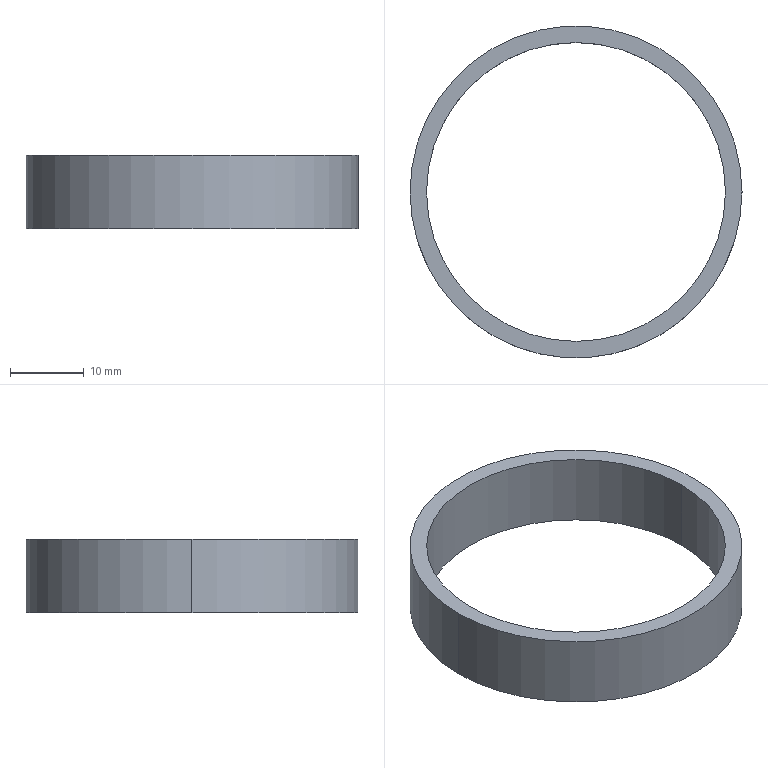Part | SolidWorks | features Extrusion 1 | 1 solid | 6 faces | box 45 x 45 x 10 mm | volume 3022 mm3 | cylinder 4 | plane 2 | commonest cylinder face diameters 40.5 x2 45 x2
STEP:
#1=CARTESIAN_POINT('',(-20.25,0.,10.));
#2=VERTEX_POINT('',#1);
#3=CARTESIAN_POINT('',(20.25,0.,10.));
#4=VERTEX_POINT('',#3);
#5=CARTESIAN_POINT('',(0.,0.,10.));
#6=DIRECTION('',(0.,0.,1.));
#7=DIRECTION('',(1.,0.,0.));
#8=AXIS2_PLACEMENT_3D('',#5,#6,#7);
#9=CIRCLE('',#8,20.25);
#10=EDGE_CURVE('',#2,#4,#9,.T.);
#11=ORIENTED_EDGE('',*,*,#10,.T.);
#12=CARTESIAN_POINT('',(20.25,0.,0.));
#13=VERTEX_POINT('',#12);
#14=CARTESIAN_POINT('',(20.25,0.,10.));
#15=DIRECTION('',(0.,0.,-1.));
#16=VECTOR('',#15,1000.);
#17=LINE('',#14,#16);
#18=EDGE_CURVE('',#4,#13,#17,.T.);
#19=ORIENTED_EDGE('',*,*,#18,.T.);
#20=CARTESIAN_POINT('',(-20.25,0.,0.));
#21=VERTEX_POINT('',#20);
#22=CARTESIAN_POINT('',(0.,0.,0.));
#23=DIRECTION('',(0.,0.,1.));
#24=DIRECTION('',(1.,0.,0.));
#25=AXIS2_PLACEMENT_3D('',#22,#23,#24);
#26=CIRCLE('',#25,20.25);
#27=EDGE_CURVE('',#21,#13,#26,.T.);
#28=ORIENTED_EDGE('',*,*,#27,.F.);
#29=CARTESIAN_POINT('',(-20.25,0.,10.));
#30=DIRECTION('',(0.,0.,-1.));
#31=VECTOR('',#30,1000.);
#32=LINE('',#29,#31);
#33=EDGE_CURVE('',#2,#21,#32,.T.);
#34=ORIENTED_EDGE('',*,*,#33,.F.);
#35=EDGE_LOOP('',(#11,#19,#28,#34));
#36=FACE_OUTER_BOUND('',#35,.T.);
#37=CARTESIAN_POINT('',(0.,0.,10.));
#38=DIRECTION('',(0.,0.,-1.));
#39=DIRECTION('',(-1.,0.,0.));
#40=AXIS2_PLACEMENT_3D('',#37,#38,#39);
#41=CYLINDRICAL_SURFACE('',#40,20.25);
#42=ADVANCED_FACE('',(#36),#41,.F.);
#43=CARTESIAN_POINT('',(22.5,0.,10.));
#44=VERTEX_POINT('',#43);
#45=CARTESIAN_POINT('',(-22.5,0.,10.));
#46=VERTEX_POINT('',#45);
#47=CARTESIAN_POINT('',(0.,0.,10.));
#48=DIRECTION('',(0.,0.,1.));
#49=DIRECTION('',(1.,0.,0.));
#50=AXIS2_PLACEMENT_3D('',#47,#48,#49);
#51=CIRCLE('',#50,22.5);
#52=EDGE_CURVE('',#44,#46,#51,.T.);
#53=ORIENTED_EDGE('',*,*,#52,.F.);
#54=CARTESIAN_POINT('',(22.5,0.,0.));
#55=VERTEX_POINT('',#54);
#56=CARTESIAN_POINT('',(22.5,0.,10.));
#57=DIRECTION('',(0.,0.,-1.));
#58=VECTOR('',#57,1000.);
#59=LINE('',#56,#58);
#60=EDGE_CURVE('',#44,#55,#59,.T.);
#61=ORIENTED_EDGE('',*,*,#60,.T.);
#62=CARTESIAN_POINT('',(-22.5,0.,0.));
#63=VERTEX_POINT('',#62);
#64=CARTESIAN_POINT('',(0.,0.,0.));
#65=DIRECTION('',(0.,0.,1.));
#66=DIRECTION('',(1.,0.,0.));
#67=AXIS2_PLACEMENT_3D('',#64,#65,#66);
#68=CIRCLE('',#67,22.5);
#69=EDGE_CURVE('',#55,#63,#68,.T.);
#70=ORIENTED_EDGE('',*,*,#69,.T.);
#71=CARTESIAN_POINT('',(-22.5,0.,10.));
#72=DIRECTION('',(0.,0.,-1.));
#73=VECTOR('',#72,1000.);
#74=LINE('',#71,#73);
#75=EDGE_CURVE('',#46,#63,#74,.T.);
#76=ORIENTED_EDGE('',*,*,#75,.F.);
#77=EDGE_LOOP('',(#53,#61,#70,#76));
#78=FACE_OUTER_BOUND('',#77,.T.);
#79=CARTESIAN_POINT('',(0.,0.,10.));
#80=DIRECTION('',(0.,0.,-1.));
#81=DIRECTION('',(-1.,0.,0.));
#82=AXIS2_PLACEMENT_3D('',#79,#80,#81);
#83=CYLINDRICAL_SURFACE('',#82,22.5);
#84=ADVANCED_FACE('',(#78),#83,.T.);
#85=CARTESIAN_POINT('',(0.,0.,10.));
#86=DIRECTION('',(0.,0.,1.));
#87=DIRECTION('',(1.,0.,0.));
#88=AXIS2_PLACEMENT_3D('',#85,#86,#87);
#89=CIRCLE('',#88,22.5);
#90=EDGE_CURVE('',#46,#44,#89,.T.);
#91=ORIENTED_EDGE('',*,*,#90,.T.);
#92=ORIENTED_EDGE('',*,*,#52,.T.);
#93=EDGE_LOOP('',(#91,#92));
#94=FACE_OUTER_BOUND('',#93,.T.);
#95=ORIENTED_EDGE('',*,*,#10,.F.);
#96=CARTESIAN_POINT('',(0.,0.,10.));
#97=DIRECTION('',(0.,0.,1.));
#98=DIRECTION('',(1.,0.,0.));
#99=AXIS2_PLACEMENT_3D('',#96,#97,#98);
#100=CIRCLE('',#99,20.25);
#101=EDGE_CURVE('',#4,#2,#100,.T.);
#102=ORIENTED_EDGE('',*,*,#101,.F.);
#103=EDGE_LOOP('',(#95,#102));
#104=FACE_BOUND('',#103,.T.);
#105=CARTESIAN_POINT('',(0.,0.,10.));
#106=DIRECTION('',(0.,0.,1.));
#107=DIRECTION('',(1.,0.,0.));
#108=AXIS2_PLACEMENT_3D('',#105,#106,#107);
#109=PLANE('',#108);
#110=ADVANCED_FACE('',(#94,#104),#109,.T.);
#111=CARTESIAN_POINT('',(0.,0.,0.));
#112=DIRECTION('',(0.,0.,1.));
#113=DIRECTION('',(1.,0.,0.));
#114=AXIS2_PLACEMENT_3D('',#111,#112,#113);
#115=CIRCLE('',#114,22.5);
#116=EDGE_CURVE('',#63,#55,#115,.T.);
#117=ORIENTED_EDGE('',*,*,#116,.F.);
#118=ORIENTED_EDGE('',*,*,#69,.F.);
#119=EDGE_LOOP('',(#117,#118));
#120=FACE_OUTER_BOUND('',#119,.T.);
#121=ORIENTED_EDGE('',*,*,#27,.T.);
#122=CARTESIAN_POINT('',(0.,0.,0.));
#123=DIRECTION('',(0.,0.,1.));
#124=DIRECTION('',(1.,0.,0.));
#125=AXIS2_PLACEMENT_3D('',#122,#123,#124);
#126=CIRCLE('',#125,20.25);
#127=EDGE_CURVE('',#13,#21,#126,.T.);
#128=ORIENTED_EDGE('',*,*,#127,.T.);
#129=EDGE_LOOP('',(#121,#128));
#130=FACE_BOUND('',#129,.T.);
#131=CARTESIAN_POINT('',(0.,0.,0.));
#132=DIRECTION('',(0.,0.,1.));
#133=DIRECTION('',(1.,0.,0.));
#134=AXIS2_PLACEMENT_3D('',#131,#132,#133);
#135=PLANE('',#134);
#136=ADVANCED_FACE('',(#120,#130),#135,.F.);
#137=ORIENTED_EDGE('',*,*,#60,.F.);
#138=ORIENTED_EDGE('',*,*,#90,.F.);
#139=ORIENTED_EDGE('',*,*,#75,.T.);
#140=ORIENTED_EDGE('',*,*,#116,.T.);
#141=EDGE_LOOP('',(#137,#138,#139,#140));
#142=FACE_OUTER_BOUND('',#141,.T.);
#143=CARTESIAN_POINT('',(0.,0.,10.));
#144=DIRECTION('',(0.,0.,-1.));
#145=DIRECTION('',(-1.,0.,0.));
#146=AXIS2_PLACEMENT_3D('',#143,#144,#145);
#147=CYLINDRICAL_SURFACE('',#146,22.5);
#148=ADVANCED_FACE('',(#142),#147,.T.);
#149=ORIENTED_EDGE('',*,*,#18,.F.);
#150=ORIENTED_EDGE('',*,*,#101,.T.);
#151=ORIENTED_EDGE('',*,*,#33,.T.);
#152=ORIENTED_EDGE('',*,*,#127,.F.);
#153=EDGE_LOOP('',(#149,#150,#151,#152));
#154=FACE_OUTER_BOUND('',#153,.T.);
#155=CARTESIAN_POINT('',(0.,0.,10.));
#156=DIRECTION('',(0.,0.,-1.));
#157=DIRECTION('',(-1.,0.,0.));
#158=AXIS2_PLACEMENT_3D('',#155,#156,#157);
#159=CYLINDRICAL_SURFACE('',#158,20.25);
#160=ADVANCED_FACE('',(#154),#159,.F.);
#161=CLOSED_SHELL('',(#42,#84,#110,#136,#148,#160));
#162=MANIFOLD_SOLID_BREP('',#161);
#163=CARTESIAN_POINT('',(0.,0.,0.));
#164=DIRECTION('',(0.,0.,1.));
#165=DIRECTION('',(1.,0.,0.));
#166=AXIS2_PLACEMENT_3D('',#163,#164,#165);
#167=(LENGTH_UNIT()NAMED_UNIT(*)SI_UNIT(.MILLI.,.METRE.));
#168=UNCERTAINTY_MEASURE_WITH_UNIT(LENGTH_MEASURE(0.00001),#167,'','');
#169=(NAMED_UNIT(*)PLANE_ANGLE_UNIT()SI_UNIT($,.RADIAN.));
#170=(NAMED_UNIT(*)SI_UNIT($,.STERADIAN.)SOLID_ANGLE_UNIT());
#171=(GEOMETRIC_REPRESENTATION_CONTEXT(3)GLOBAL_UNCERTAINTY_ASSIGNED_CONTEXT((#168))GLOBAL_UNIT_ASSIGNED_CONTEXT((#167,#169,#170))REPRESENTATION_CONTEXT('',''));
#172=ADVANCED_BREP_SHAPE_REPRESENTATION('',(#162,#166),#171);